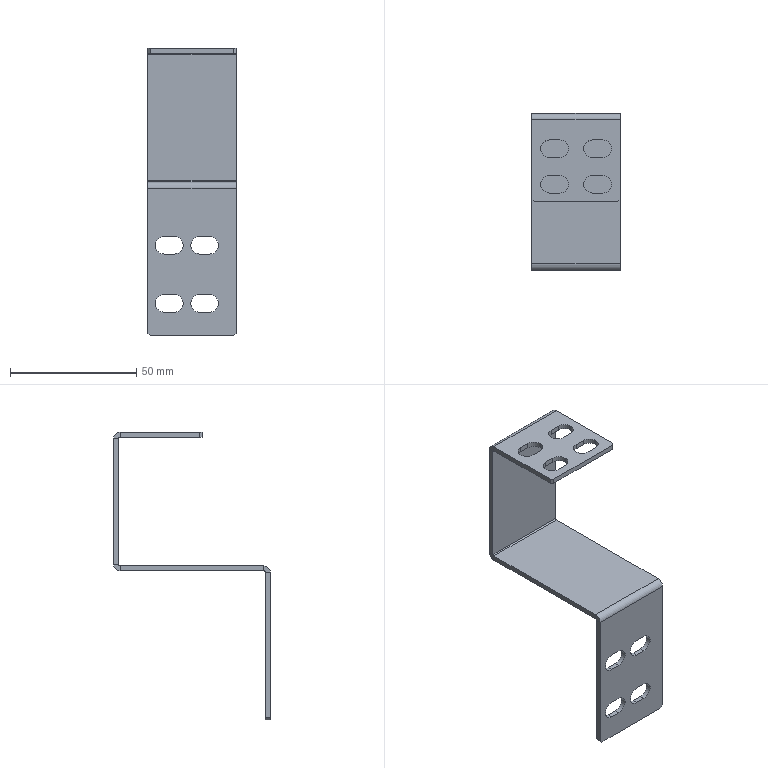Part | SolidWorks | features EdgeFlange 3, HoleWzd 2, Chamfer 1, FlatPattern 1, SMBaseFlange 1, SheetMetal 1 | 1 solid | 70 faces | box 35 x 62 x 114 mm | volume 13287 mm3 | plane 44 | cylinder 26 | commonest cylinder face diameters 7 x20 1 x3 5 x3